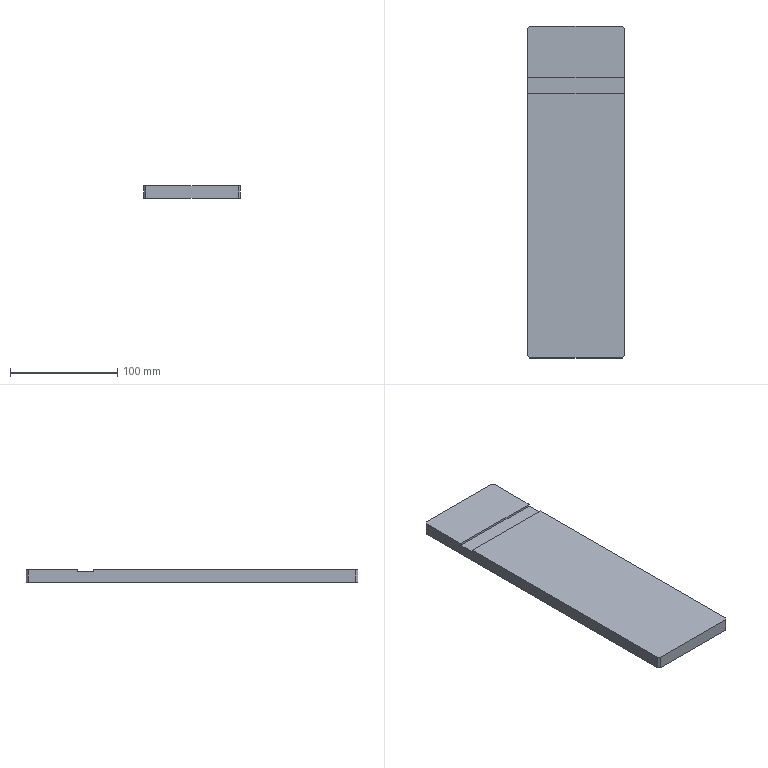Part | STEP file | 001-005-Shaft threading fixture vertical plate | 1 solid | 14 faces | box 90 x 310 x 12 mm | volume 332004 mm3 | plane 14
STEP:
#1=CARTESIAN_POINT('',(0.,0.,0.));
#2=DIRECTION('',(0.,0.,1.));
#3=DIRECTION('',(1.,0.,0.));
#4=AXIS2_PLACEMENT_3D('',#1,#2,#3);
#5=CARTESIAN_POINT('',(-45.,153.,12.));
#6=VERTEX_POINT('',#5);
#7=CARTESIAN_POINT('',(-45.,107.,12.));
#8=VERTEX_POINT('',#7);
#9=CARTESIAN_POINT('',(-45.,-155.,12.));
#10=DIRECTION('',(0.,-1.,0.));
#11=VECTOR('',#10,1.);
#12=LINE('',#9,#11);
#13=CARTESIAN_POINT('',(0.,0.,12.));
#14=DIRECTION('',(0.,0.,-1.));
#15=DIRECTION('',(-1.,0.,0.));
#16=AXIS2_PLACEMENT_3D('',#13,#14,#15);
#17=PLANE('',#16);
#18=CARTESIAN_POINT('',(45.,-155.));
#19=DIRECTION('',(0.,-1.));
#20=VECTOR('',#19,1.);
#21=LINE('',#18,#20);
#22=(GEOMETRIC_REPRESENTATION_CONTEXT(2)PARAMETRIC_REPRESENTATION_CONTEXT()REPRESENTATION_CONTEXT('',''));
#23=DEFINITIONAL_REPRESENTATION('',(#21),#22);
#24=PCURVE('',#17,#23);
#25=CARTESIAN_POINT('',(-45.,-155.,12.));
#26=DIRECTION('',(1.,0.,0.));
#27=DIRECTION('',(0.,1.,0.));
#28=AXIS2_PLACEMENT_3D('',#25,#26,#27);
#29=PLANE('',#28);
#30=CARTESIAN_POINT('',(0.,0.));
#31=DIRECTION('',(-1.,0.));
#32=VECTOR('',#31,1.);
#33=LINE('',#30,#32);
#34=(GEOMETRIC_REPRESENTATION_CONTEXT(2)PARAMETRIC_REPRESENTATION_CONTEXT()REPRESENTATION_CONTEXT('',''));
#35=DEFINITIONAL_REPRESENTATION('',(#33),#34);
#36=PCURVE('',#29,#35);
#37=SURFACE_CURVE('',#12,(#24,#36),.PCURVE_S1.);
#38=EDGE_CURVE('',#6,#8,#37,.T.);
#39=ORIENTED_EDGE('',*,*,#38,.T.);
#40=CARTESIAN_POINT('',(45.,107.,12.));
#41=VERTEX_POINT('',#40);
#42=CARTESIAN_POINT('',(-45.,107.,12.));
#43=DIRECTION('',(1.,0.,0.));
#44=VECTOR('',#43,1.);
#45=LINE('',#42,#44);
#46=CARTESIAN_POINT('',(45.,107.));
#47=DIRECTION('',(-1.,0.));
#48=VECTOR('',#47,1.);
#49=LINE('',#46,#48);
#50=(GEOMETRIC_REPRESENTATION_CONTEXT(2)PARAMETRIC_REPRESENTATION_CONTEXT()REPRESENTATION_CONTEXT('',''));
#51=DEFINITIONAL_REPRESENTATION('',(#49),#50);
#52=PCURVE('',#17,#51);
#53=CARTESIAN_POINT('',(-45.,107.,12.));
#54=DIRECTION('',(0.,1.,0.));
#55=DIRECTION('',(0.,0.,1.));
#56=AXIS2_PLACEMENT_3D('',#53,#54,#55);
#57=PLANE('',#56);
#58=CARTESIAN_POINT('',(0.,0.));
#59=DIRECTION('',(0.,1.));
#60=VECTOR('',#59,1.);
#61=LINE('',#58,#60);
#62=(GEOMETRIC_REPRESENTATION_CONTEXT(2)PARAMETRIC_REPRESENTATION_CONTEXT()REPRESENTATION_CONTEXT('',''));
#63=DEFINITIONAL_REPRESENTATION('',(#61),#62);
#64=PCURVE('',#57,#63);
#65=SURFACE_CURVE('',#45,(#52,#64),.PCURVE_S1.);
#66=EDGE_CURVE('',#8,#41,#65,.T.);
#67=ORIENTED_EDGE('',*,*,#66,.T.);
#68=CARTESIAN_POINT('',(45.,153.,12.));
#69=VERTEX_POINT('',#68);
#70=CARTESIAN_POINT('',(45.,-155.,12.));
#71=DIRECTION('',(0.,1.,0.));
#72=VECTOR('',#71,1.);
#73=LINE('',#70,#72);
#74=CARTESIAN_POINT('',(-45.,-155.));
#75=DIRECTION('',(0.,1.));
#76=VECTOR('',#75,1.);
#77=LINE('',#74,#76);
#78=(GEOMETRIC_REPRESENTATION_CONTEXT(2)PARAMETRIC_REPRESENTATION_CONTEXT()REPRESENTATION_CONTEXT('',''));
#79=DEFINITIONAL_REPRESENTATION('',(#77),#78);
#80=PCURVE('',#17,#79);
#81=CARTESIAN_POINT('',(45.,-155.,12.));
#82=DIRECTION('',(-1.,0.,0.));
#83=DIRECTION('',(0.,-1.,0.));
#84=AXIS2_PLACEMENT_3D('',#81,#82,#83);
#85=PLANE('',#84);
#86=CARTESIAN_POINT('',(0.,0.));
#87=DIRECTION('',(-1.,0.));
#88=VECTOR('',#87,1.);
#89=LINE('',#86,#88);
#90=(GEOMETRIC_REPRESENTATION_CONTEXT(2)PARAMETRIC_REPRESENTATION_CONTEXT()REPRESENTATION_CONTEXT('',''));
#91=DEFINITIONAL_REPRESENTATION('',(#89),#90);
#92=PCURVE('',#85,#91);
#93=SURFACE_CURVE('',#73,(#80,#92),.PCURVE_S1.);
#94=EDGE_CURVE('',#41,#69,#93,.T.);
#95=ORIENTED_EDGE('',*,*,#94,.T.);
#96=CARTESIAN_POINT('',(43.,155.,12.));
#97=VERTEX_POINT('',#96);
#98=CARTESIAN_POINT('',(43.,155.,12.));
#99=DIRECTION('',(-0.7071,0.7071,0.));
#100=VECTOR('',#99,1.);
#101=LINE('',#98,#100);
#102=CARTESIAN_POINT('',(-43.,155.));
#103=DIRECTION('',(0.7071,0.7071));
#104=VECTOR('',#103,1.);
#105=LINE('',#102,#104);
#106=(GEOMETRIC_REPRESENTATION_CONTEXT(2)PARAMETRIC_REPRESENTATION_CONTEXT()REPRESENTATION_CONTEXT('',''));
#107=DEFINITIONAL_REPRESENTATION('',(#105),#106);
#108=PCURVE('',#17,#107);
#109=CARTESIAN_POINT('',(43.,155.,12.));
#110=DIRECTION('',(-0.7071,-0.7071,0.));
#111=DIRECTION('',(0.,0.,-1.));
#112=AXIS2_PLACEMENT_3D('',#109,#110,#111);
#113=PLANE('',#112);
#114=CARTESIAN_POINT('',(0.,0.));
#115=DIRECTION('',(0.,-1.));
#116=VECTOR('',#115,1.);
#117=LINE('',#114,#116);
#118=(GEOMETRIC_REPRESENTATION_CONTEXT(2)PARAMETRIC_REPRESENTATION_CONTEXT()REPRESENTATION_CONTEXT('',''));
#119=DEFINITIONAL_REPRESENTATION('',(#117),#118);
#120=PCURVE('',#113,#119);
#121=SURFACE_CURVE('',#101,(#108,#120),.PCURVE_S1.);
#122=EDGE_CURVE('',#69,#97,#121,.T.);
#123=ORIENTED_EDGE('',*,*,#122,.T.);
#124=CARTESIAN_POINT('',(-43.,155.,12.));
#125=VERTEX_POINT('',#124);
#126=CARTESIAN_POINT('',(-45.,155.,12.));
#127=DIRECTION('',(-1.,0.,0.));
#128=VECTOR('',#127,1.);
#129=LINE('',#126,#128);
#130=CARTESIAN_POINT('',(45.,155.));
#131=DIRECTION('',(1.,0.));
#132=VECTOR('',#131,1.);
#133=LINE('',#130,#132);
#134=(GEOMETRIC_REPRESENTATION_CONTEXT(2)PARAMETRIC_REPRESENTATION_CONTEXT()REPRESENTATION_CONTEXT('',''));
#135=DEFINITIONAL_REPRESENTATION('',(#133),#134);
#136=PCURVE('',#17,#135);
#137=CARTESIAN_POINT('',(-45.,155.,12.));
#138=DIRECTION('',(0.,-1.,0.));
#139=DIRECTION('',(0.,0.,-1.));
#140=AXIS2_PLACEMENT_3D('',#137,#138,#139);
#141=PLANE('',#140);
#142=CARTESIAN_POINT('',(0.,0.));
#143=DIRECTION('',(0.,-1.));
#144=VECTOR('',#143,1.);
#145=LINE('',#142,#144);
#146=(GEOMETRIC_REPRESENTATION_CONTEXT(2)PARAMETRIC_REPRESENTATION_CONTEXT()REPRESENTATION_CONTEXT('',''));
#147=DEFINITIONAL_REPRESENTATION('',(#145),#146);
#148=PCURVE('',#141,#147);
#149=SURFACE_CURVE('',#129,(#136,#148),.PCURVE_S1.);
#150=EDGE_CURVE('',#97,#125,#149,.T.);
#151=ORIENTED_EDGE('',*,*,#150,.T.);
#152=CARTESIAN_POINT('',(-45.,153.,12.));
#153=DIRECTION('',(-0.7071,-0.7071,0.));
#154=VECTOR('',#153,1.);
#155=LINE('',#152,#154);
#156=CARTESIAN_POINT('',(45.,153.));
#157=DIRECTION('',(0.7071,-0.7071));
#158=VECTOR('',#157,1.);
#159=LINE('',#156,#158);
#160=(GEOMETRIC_REPRESENTATION_CONTEXT(2)PARAMETRIC_REPRESENTATION_CONTEXT()REPRESENTATION_CONTEXT('',''));
#161=DEFINITIONAL_REPRESENTATION('',(#159),#160);
#162=PCURVE('',#17,#161);
#163=CARTESIAN_POINT('',(-45.,153.,12.));
#164=DIRECTION('',(0.7071,-0.7071,0.));
#165=DIRECTION('',(0.,0.,-1.));
#166=AXIS2_PLACEMENT_3D('',#163,#164,#165);
#167=PLANE('',#166);
#168=CARTESIAN_POINT('',(0.,0.));
#169=DIRECTION('',(0.,-1.));
#170=VECTOR('',#169,1.);
#171=LINE('',#168,#170);
#172=(GEOMETRIC_REPRESENTATION_CONTEXT(2)PARAMETRIC_REPRESENTATION_CONTEXT()REPRESENTATION_CONTEXT('',''));
#173=DEFINITIONAL_REPRESENTATION('',(#171),#172);
#174=PCURVE('',#167,#173);
#175=SURFACE_CURVE('',#155,(#162,#174),.PCURVE_S1.);
#176=EDGE_CURVE('',#125,#6,#175,.T.);
#177=ORIENTED_EDGE('',*,*,#176,.T.);
#178=EDGE_LOOP('',(#39,#67,#95,#123,#151,#177));
#179=FACE_BOUND('',#178,.T.);
#180=ADVANCED_FACE('',(#179),#17,.F.);
#181=ORIENTED_EDGE('',*,*,#94,.F.);
#182=CARTESIAN_POINT('',(45.,107.,10.));
#183=VERTEX_POINT('',#182);
#184=CARTESIAN_POINT('',(45.,107.,12.));
#185=DIRECTION('',(0.,0.,1.));
#186=VECTOR('',#185,1.);
#187=LINE('',#184,#186);
#188=CARTESIAN_POINT('',(-262.,0.));
#189=DIRECTION('',(0.,1.));
#190=VECTOR('',#189,1.);
#191=LINE('',#188,#190);
#192=(GEOMETRIC_REPRESENTATION_CONTEXT(2)PARAMETRIC_REPRESENTATION_CONTEXT()REPRESENTATION_CONTEXT('',''));
#193=DEFINITIONAL_REPRESENTATION('',(#191),#192);
#194=PCURVE('',#85,#193);
#195=CARTESIAN_POINT('',(0.,90.));
#196=DIRECTION('',(1.,0.));
#197=VECTOR('',#196,1.);
#198=LINE('',#195,#197);
#199=(GEOMETRIC_REPRESENTATION_CONTEXT(2)PARAMETRIC_REPRESENTATION_CONTEXT()REPRESENTATION_CONTEXT('',''));
#200=DEFINITIONAL_REPRESENTATION('',(#198),#199);
#201=PCURVE('',#57,#200);
#202=SURFACE_CURVE('',#187,(#194,#201),.PCURVE_S1.);
#203=EDGE_CURVE('',#183,#41,#202,.T.);
#204=ORIENTED_EDGE('',*,*,#203,.F.);
#205=CARTESIAN_POINT('',(45.,92.,10.));
#206=VERTEX_POINT('',#205);
#207=CARTESIAN_POINT('',(45.,107.,10.));
#208=DIRECTION('',(0.,1.,0.));
#209=VECTOR('',#208,1.);
#210=LINE('',#207,#209);
#211=CARTESIAN_POINT('',(-262.,-2.));
#212=DIRECTION('',(-1.,0.));
#213=VECTOR('',#212,1.);
#214=LINE('',#211,#213);
#215=(GEOMETRIC_REPRESENTATION_CONTEXT(2)PARAMETRIC_REPRESENTATION_CONTEXT()REPRESENTATION_CONTEXT('',''));
#216=DEFINITIONAL_REPRESENTATION('',(#214),#215);
#217=PCURVE('',#85,#216);
#218=CARTESIAN_POINT('',(-45.,107.,10.));
#219=DIRECTION('',(0.,0.,-1.));
#220=DIRECTION('',(0.,1.,0.));
#221=AXIS2_PLACEMENT_3D('',#218,#219,#220);
#222=PLANE('',#221);
#223=CARTESIAN_POINT('',(0.,90.));
#224=DIRECTION('',(1.,0.));
#225=VECTOR('',#224,1.);
#226=LINE('',#223,#225);
#227=(GEOMETRIC_REPRESENTATION_CONTEXT(2)PARAMETRIC_REPRESENTATION_CONTEXT()REPRESENTATION_CONTEXT('',''));
#228=DEFINITIONAL_REPRESENTATION('',(#226),#227);
#229=PCURVE('',#222,#228);
#230=SURFACE_CURVE('',#210,(#217,#229),.PCURVE_S1.);
#231=EDGE_CURVE('',#206,#183,#230,.T.);
#232=ORIENTED_EDGE('',*,*,#231,.F.);
#233=CARTESIAN_POINT('',(45.,92.,12.));
#234=VERTEX_POINT('',#233);
#235=CARTESIAN_POINT('',(45.,92.,12.));
#236=DIRECTION('',(0.,0.,-1.));
#237=VECTOR('',#236,1.);
#238=LINE('',#235,#237);
#239=CARTESIAN_POINT('',(-247.,0.));
#240=DIRECTION('',(0.,-1.));
#241=VECTOR('',#240,1.);
#242=LINE('',#239,#241);
#243=(GEOMETRIC_REPRESENTATION_CONTEXT(2)PARAMETRIC_REPRESENTATION_CONTEXT()REPRESENTATION_CONTEXT('',''));
#244=DEFINITIONAL_REPRESENTATION('',(#242),#243);
#245=PCURVE('',#85,#244);
#246=CARTESIAN_POINT('',(-45.,92.,12.));
#247=DIRECTION('',(0.,-1.,0.));
#248=DIRECTION('',(1.,0.,0.));
#249=AXIS2_PLACEMENT_3D('',#246,#247,#248);
#250=PLANE('',#249);
#251=CARTESIAN_POINT('',(90.,0.));
#252=DIRECTION('',(0.,-1.));
#253=VECTOR('',#252,1.);
#254=LINE('',#251,#253);
#255=(GEOMETRIC_REPRESENTATION_CONTEXT(2)PARAMETRIC_REPRESENTATION_CONTEXT()REPRESENTATION_CONTEXT('',''));
#256=DEFINITIONAL_REPRESENTATION('',(#254),#255);
#257=PCURVE('',#250,#256);
#258=SURFACE_CURVE('',#238,(#245,#257),.PCURVE_S1.);
#259=EDGE_CURVE('',#234,#206,#258,.T.);
#260=ORIENTED_EDGE('',*,*,#259,.F.);
#261=CARTESIAN_POINT('',(45.,-153.,12.));
#262=VERTEX_POINT('',#261);
#263=CARTESIAN_POINT('',(45.,-155.,12.));
#264=DIRECTION('',(0.,1.,0.));
#265=VECTOR('',#264,1.);
#266=LINE('',#263,#265);
#267=CARTESIAN_POINT('',(0.,0.));
#268=DIRECTION('',(-1.,0.));
#269=VECTOR('',#268,1.);
#270=LINE('',#267,#269);
#271=(GEOMETRIC_REPRESENTATION_CONTEXT(2)PARAMETRIC_REPRESENTATION_CONTEXT()REPRESENTATION_CONTEXT('',''));
#272=DEFINITIONAL_REPRESENTATION('',(#270),#271);
#273=PCURVE('',#85,#272);
#274=CARTESIAN_POINT('',(0.,0.,12.));
#275=DIRECTION('',(0.,0.,-1.));
#276=DIRECTION('',(-1.,0.,0.));
#277=AXIS2_PLACEMENT_3D('',#274,#275,#276);
#278=PLANE('',#277);
#279=CARTESIAN_POINT('',(-45.,-155.));
#280=DIRECTION('',(0.,1.));
#281=VECTOR('',#280,1.);
#282=LINE('',#279,#281);
#283=(GEOMETRIC_REPRESENTATION_CONTEXT(2)PARAMETRIC_REPRESENTATION_CONTEXT()REPRESENTATION_CONTEXT('',''));
#284=DEFINITIONAL_REPRESENTATION('',(#282),#283);
#285=PCURVE('',#278,#284);
#286=SURFACE_CURVE('',#266,(#273,#285),.PCURVE_S1.);
#287=EDGE_CURVE('',#262,#234,#286,.T.);
#288=ORIENTED_EDGE('',*,*,#287,.F.);
#289=CARTESIAN_POINT('',(45.,-153.,0.));
#290=VERTEX_POINT('',#289);
#291=CARTESIAN_POINT('',(45.,-153.,12.));
#292=DIRECTION('',(0.,0.,-1.));
#293=VECTOR('',#292,1.);
#294=LINE('',#291,#293);
#295=CARTESIAN_POINT('',(-2.,0.));
#296=DIRECTION('',(0.,-1.));
#297=VECTOR('',#296,1.);
#298=LINE('',#295,#297);
#299=(GEOMETRIC_REPRESENTATION_CONTEXT(2)PARAMETRIC_REPRESENTATION_CONTEXT()REPRESENTATION_CONTEXT('',''));
#300=DEFINITIONAL_REPRESENTATION('',(#298),#299);
#301=PCURVE('',#85,#300);
#302=CARTESIAN_POINT('',(45.,-153.,12.));
#303=DIRECTION('',(-0.7071,0.7071,0.));
#304=DIRECTION('',(0.,0.,-1.));
#305=AXIS2_PLACEMENT_3D('',#302,#303,#304);
#306=PLANE('',#305);
#307=CARTESIAN_POINT('',(0.,0.));
#308=DIRECTION('',(1.,0.));
#309=VECTOR('',#308,1.);
#310=LINE('',#307,#309);
#311=(GEOMETRIC_REPRESENTATION_CONTEXT(2)PARAMETRIC_REPRESENTATION_CONTEXT()REPRESENTATION_CONTEXT('',''));
#312=DEFINITIONAL_REPRESENTATION('',(#310),#311);
#313=PCURVE('',#306,#312);
#314=SURFACE_CURVE('',#294,(#301,#313),.PCURVE_S1.);
#315=EDGE_CURVE('',#262,#290,#314,.T.);
#316=ORIENTED_EDGE('',*,*,#315,.T.);
#317=CARTESIAN_POINT('',(45.,153.,0.));
#318=VERTEX_POINT('',#317);
#319=CARTESIAN_POINT('',(45.,-155.,0.));
#320=DIRECTION('',(0.,1.,0.));
#321=VECTOR('',#320,1.);
#322=LINE('',#319,#321);
#323=CARTESIAN_POINT('',(0.,-12.));
#324=DIRECTION('',(-1.,0.));
#325=VECTOR('',#324,1.);
#326=LINE('',#323,#325);
#327=(GEOMETRIC_REPRESENTATION_CONTEXT(2)PARAMETRIC_REPRESENTATION_CONTEXT()REPRESENTATION_CONTEXT('',''));
#328=DEFINITIONAL_REPRESENTATION('',(#326),#327);
#329=PCURVE('',#85,#328);
#330=CARTESIAN_POINT('',(0.,0.,0.));
#331=DIRECTION('',(0.,0.,-1.));
#332=DIRECTION('',(-1.,0.,0.));
#333=AXIS2_PLACEMENT_3D('',#330,#331,#332);
#334=PLANE('',#333);
#335=CARTESIAN_POINT('',(-45.,-155.));
#336=DIRECTION('',(0.,1.));
#337=VECTOR('',#336,1.);
#338=LINE('',#335,#337);
#339=(GEOMETRIC_REPRESENTATION_CONTEXT(2)PARAMETRIC_REPRESENTATION_CONTEXT()REPRESENTATION_CONTEXT('',''));
#340=DEFINITIONAL_REPRESENTATION('',(#338),#339);
#341=PCURVE('',#334,#340);
#342=SURFACE_CURVE('',#322,(#329,#341),.PCURVE_S1.);
#343=EDGE_CURVE('',#290,#318,#342,.T.);
#344=ORIENTED_EDGE('',*,*,#343,.T.);
#345=CARTESIAN_POINT('',(45.,153.,12.));
#346=DIRECTION('',(0.,0.,1.));
#347=VECTOR('',#346,1.);
#348=LINE('',#345,#347);
#349=CARTESIAN_POINT('',(-308.,0.));
#350=DIRECTION('',(0.,1.));
#351=VECTOR('',#350,1.);
#352=LINE('',#349,#351);
#353=(GEOMETRIC_REPRESENTATION_CONTEXT(2)PARAMETRIC_REPRESENTATION_CONTEXT()REPRESENTATION_CONTEXT('',''));
#354=DEFINITIONAL_REPRESENTATION('',(#352),#353);
#355=PCURVE('',#85,#354);
#356=CARTESIAN_POINT('',(0.,2.828));
#357=DIRECTION('',(-1.,0.));
#358=VECTOR('',#357,1.);
#359=LINE('',#356,#358);
#360=(GEOMETRIC_REPRESENTATION_CONTEXT(2)PARAMETRIC_REPRESENTATION_CONTEXT()REPRESENTATION_CONTEXT('',''));
#361=DEFINITIONAL_REPRESENTATION('',(#359),#360);
#362=PCURVE('',#113,#361);
#363=SURFACE_CURVE('',#348,(#355,#362),.PCURVE_S1.);
#364=EDGE_CURVE('',#318,#69,#363,.T.);
#365=ORIENTED_EDGE('',*,*,#364,.T.);
#366=EDGE_LOOP('',(#181,#204,#232,#260,#288,#316,#344,#365));
#367=FACE_BOUND('',#366,.T.);
#368=ADVANCED_FACE('',(#367),#85,.F.);
#369=CARTESIAN_POINT('',(43.,155.,0.));
#370=VERTEX_POINT('',#369);
#371=CARTESIAN_POINT('',(-43.,155.,0.));
#372=VERTEX_POINT('',#371);
#373=CARTESIAN_POINT('',(-45.,155.,0.));
#374=DIRECTION('',(-1.,0.,0.));
#375=VECTOR('',#374,1.);
#376=LINE('',#373,#375);
#377=CARTESIAN_POINT('',(12.,0.));
#378=DIRECTION('',(0.,-1.));
#379=VECTOR('',#378,1.);
#380=LINE('',#377,#379);
#381=(GEOMETRIC_REPRESENTATION_CONTEXT(2)PARAMETRIC_REPRESENTATION_CONTEXT()REPRESENTATION_CONTEXT('',''));
#382=DEFINITIONAL_REPRESENTATION('',(#380),#381);
#383=PCURVE('',#141,#382);
#384=CARTESIAN_POINT('',(45.,155.));
#385=DIRECTION('',(1.,0.));
#386=VECTOR('',#385,1.);
#387=LINE('',#384,#386);
#388=(GEOMETRIC_REPRESENTATION_CONTEXT(2)PARAMETRIC_REPRESENTATION_CONTEXT()REPRESENTATION_CONTEXT('',''));
#389=DEFINITIONAL_REPRESENTATION('',(#387),#388);
#390=PCURVE('',#334,#389);
#391=SURFACE_CURVE('',#376,(#383,#390),.PCURVE_S1.);
#392=EDGE_CURVE('',#370,#372,#391,.T.);
#393=ORIENTED_EDGE('',*,*,#392,.T.);
#394=CARTESIAN_POINT('',(-43.,155.,12.));
#395=DIRECTION('',(0.,0.,1.));
#396=VECTOR('',#395,1.);
#397=LINE('',#394,#396);
#398=CARTESIAN_POINT('',(0.,2.));
#399=DIRECTION('',(-1.,0.));
#400=VECTOR('',#399,1.);
#401=LINE('',#398,#400);
#402=(GEOMETRIC_REPRESENTATION_CONTEXT(2)PARAMETRIC_REPRESENTATION_CONTEXT()REPRESENTATION_CONTEXT('',''));
#403=DEFINITIONAL_REPRESENTATION('',(#401),#402);
#404=PCURVE('',#141,#403);
#405=CARTESIAN_POINT('',(0.,2.828));
#406=DIRECTION('',(-1.,0.));
#407=VECTOR('',#406,1.);
#408=LINE('',#405,#407);
#409=(GEOMETRIC_REPRESENTATION_CONTEXT(2)PARAMETRIC_REPRESENTATION_CONTEXT()REPRESENTATION_CONTEXT('',''));
#410=DEFINITIONAL_REPRESENTATION('',(#408),#409);
#411=PCURVE('',#167,#410);
#412=SURFACE_CURVE('',#397,(#404,#411),.PCURVE_S1.);
#413=EDGE_CURVE('',#372,#125,#412,.T.);
#414=ORIENTED_EDGE('',*,*,#413,.T.);
#415=ORIENTED_EDGE('',*,*,#150,.F.);
#416=CARTESIAN_POINT('',(43.,155.,12.));
#417=DIRECTION('',(0.,0.,-1.));
#418=VECTOR('',#417,1.);
#419=LINE('',#416,#418);
#420=CARTESIAN_POINT('',(0.,88.));
#421=DIRECTION('',(1.,0.));
#422=VECTOR('',#421,1.);
#423=LINE('',#420,#422);
#424=(GEOMETRIC_REPRESENTATION_CONTEXT(2)PARAMETRIC_REPRESENTATION_CONTEXT()REPRESENTATION_CONTEXT('',''));
#425=DEFINITIONAL_REPRESENTATION('',(#423),#424);
#426=PCURVE('',#141,#425);
#427=CARTESIAN_POINT('',(0.,0.));
#428=DIRECTION('',(1.,0.));
#429=VECTOR('',#428,1.);
#430=LINE('',#427,#429);
#431=(GEOMETRIC_REPRESENTATION_CONTEXT(2)PARAMETRIC_REPRESENTATION_CONTEXT()REPRESENTATION_CONTEXT('',''));
#432=DEFINITIONAL_REPRESENTATION('',(#430),#431);
#433=PCURVE('',#113,#432);
#434=SURFACE_CURVE('',#419,(#426,#433),.PCURVE_S1.);
#435=EDGE_CURVE('',#97,#370,#434,.T.);
#436=ORIENTED_EDGE('',*,*,#435,.T.);
#437=EDGE_LOOP('',(#393,#414,#415,#436));
#438=FACE_BOUND('',#437,.T.);
#439=ADVANCED_FACE('',(#438),#141,.F.);
#440=CARTESIAN_POINT('',(-45.,92.,10.));
#441=VERTEX_POINT('',#440);
#442=CARTESIAN_POINT('',(-45.,107.,10.));
#443=VERTEX_POINT('',#442);
#444=CARTESIAN_POINT('',(-45.,107.,10.));
#445=DIRECTION('',(0.,1.,0.));
#446=VECTOR('',#445,1.);
#447=LINE('',#444,#446);
#448=CARTESIAN_POINT('',(262.,-2.));
#449=DIRECTION('',(1.,0.));
#450=VECTOR('',#449,1.);
#451=LINE('',#448,#450);
#452=(GEOMETRIC_REPRESENTATION_CONTEXT(2)PARAMETRIC_REPRESENTATION_CONTEXT()REPRESENTATION_CONTEXT('',''));
#453=DEFINITIONAL_REPRESENTATION('',(#451),#452);
#454=PCURVE('',#29,#453);
#455=CARTESIAN_POINT('',(0.,0.));
#456=DIRECTION('',(1.,0.));
#457=VECTOR('',#456,1.);
#458=LINE('',#455,#457);
#459=(GEOMETRIC_REPRESENTATION_CONTEXT(2)PARAMETRIC_REPRESENTATION_CONTEXT()REPRESENTATION_CONTEXT('',''));
#460=DEFINITIONAL_REPRESENTATION('',(#458),#459);
#461=PCURVE('',#222,#460);
#462=SURFACE_CURVE('',#447,(#454,#461),.PCURVE_S1.);
#463=EDGE_CURVE('',#441,#443,#462,.T.);
#464=ORIENTED_EDGE('',*,*,#463,.T.);
#465=CARTESIAN_POINT('',(-45.,107.,12.));
#466=DIRECTION('',(0.,0.,1.));
#467=VECTOR('',#466,1.);
#468=LINE('',#465,#467);
#469=CARTESIAN_POINT('',(262.,0.));
#470=DIRECTION('',(0.,1.));
#471=VECTOR('',#470,1.);
#472=LINE('',#469,#471);
#473=(GEOMETRIC_REPRESENTATION_CONTEXT(2)PARAMETRIC_REPRESENTATION_CONTEXT()REPRESENTATION_CONTEXT('',''));
#474=DEFINITIONAL_REPRESENTATION('',(#472),#473);
#475=PCURVE('',#29,#474);
#476=CARTESIAN_POINT('',(0.,0.));
#477=DIRECTION('',(1.,0.));
#478=VECTOR('',#477,1.);
#479=LINE('',#476,#478);
#480=(GEOMETRIC_REPRESENTATION_CONTEXT(2)PARAMETRIC_REPRESENTATION_CONTEXT()REPRESENTATION_CONTEXT('',''));
#481=DEFINITIONAL_REPRESENTATION('',(#479),#480);
#482=PCURVE('',#57,#481);
#483=SURFACE_CURVE('',#468,(#475,#482),.PCURVE_S1.);
#484=EDGE_CURVE('',#443,#8,#483,.T.);
#485=ORIENTED_EDGE('',*,*,#484,.T.);
#486=ORIENTED_EDGE('',*,*,#38,.F.);
#487=CARTESIAN_POINT('',(-45.,153.,0.));
#488=VERTEX_POINT('',#487);
#489=CARTESIAN_POINT('',(-45.,153.,12.));
#490=DIRECTION('',(0.,0.,-1.));
#491=VECTOR('',#490,1.);
#492=LINE('',#489,#491);
#493=CARTESIAN_POINT('',(308.,0.));
#494=DIRECTION('',(0.,-1.));
#495=VECTOR('',#494,1.);
#496=LINE('',#493,#495);
#497=(GEOMETRIC_REPRESENTATION_CONTEXT(2)PARAMETRIC_REPRESENTATION_CONTEXT()REPRESENTATION_CONTEXT('',''));
#498=DEFINITIONAL_REPRESENTATION('',(#496),#497);
#499=PCURVE('',#29,#498);
#500=CARTESIAN_POINT('',(0.,0.));
#501=DIRECTION('',(1.,0.));
#502=VECTOR('',#501,1.);
#503=LINE('',#500,#502);
#504=(GEOMETRIC_REPRESENTATION_CONTEXT(2)PARAMETRIC_REPRESENTATION_CONTEXT()REPRESENTATION_CONTEXT('',''));
#505=DEFINITIONAL_REPRESENTATION('',(#503),#504);
#506=PCURVE('',#167,#505);
#507=SURFACE_CURVE('',#492,(#499,#506),.PCURVE_S1.);
#508=EDGE_CURVE('',#6,#488,#507,.T.);
#509=ORIENTED_EDGE('',*,*,#508,.T.);
#510=CARTESIAN_POINT('',(-45.,-153.,0.));
#511=VERTEX_POINT('',#510);
#512=CARTESIAN_POINT('',(-45.,-155.,0.));
#513=DIRECTION('',(0.,-1.,0.));
#514=VECTOR('',#513,1.);
#515=LINE('',#512,#514);
#516=CARTESIAN_POINT('',(0.,-12.));
#517=DIRECTION('',(-1.,0.));
#518=VECTOR('',#517,1.);
#519=LINE('',#516,#518);
#520=(GEOMETRIC_REPRESENTATION_CONTEXT(2)PARAMETRIC_REPRESENTATION_CONTEXT()REPRESENTATION_CONTEXT('',''));
#521=DEFINITIONAL_REPRESENTATION('',(#519),#520);
#522=PCURVE('',#29,#521);
#523=CARTESIAN_POINT('',(45.,-155.));
#524=DIRECTION('',(0.,-1.));
#525=VECTOR('',#524,1.);
#526=LINE('',#523,#525);
#527=(GEOMETRIC_REPRESENTATION_CONTEXT(2)PARAMETRIC_REPRESENTATION_CONTEXT()REPRESENTATION_CONTEXT('',''));
#528=DEFINITIONAL_REPRESENTATION('',(#526),#527);
#529=PCURVE('',#334,#528);
#530=SURFACE_CURVE('',#515,(#522,#529),.PCURVE_S1.);
#531=EDGE_CURVE('',#488,#511,#530,.T.);
#532=ORIENTED_EDGE('',*,*,#531,.T.);
#533=CARTESIAN_POINT('',(-45.,-153.,12.));
#534=VERTEX_POINT('',#533);
#535=CARTESIAN_POINT('',(-45.,-153.,12.));
#536=DIRECTION('',(0.,0.,1.));
#537=VECTOR('',#536,1.);
#538=LINE('',#535,#537);
#539=CARTESIAN_POINT('',(2.,0.));
#540=DIRECTION('',(0.,1.));
#541=VECTOR('',#540,1.);
#542=LINE('',#539,#541);
#543=(GEOMETRIC_REPRESENTATION_CONTEXT(2)PARAMETRIC_REPRESENTATION_CONTEXT()REPRESENTATION_CONTEXT('',''));
#544=DEFINITIONAL_REPRESENTATION('',(#542),#543);
#545=PCURVE('',#29,#544);
#546=CARTESIAN_POINT('',(-43.,-155.,12.));
#547=DIRECTION('',(0.7071,0.7071,0.));
#548=DIRECTION('',(0.,0.,-1.));
#549=AXIS2_PLACEMENT_3D('',#546,#547,#548);
#550=PLANE('',#549);
#551=CARTESIAN_POINT('',(0.,2.828));
#552=DIRECTION('',(-1.,0.));
#553=VECTOR('',#552,1.);
#554=LINE('',#551,#553);
#555=(GEOMETRIC_REPRESENTATION_CONTEXT(2)PARAMETRIC_REPRESENTATION_CONTEXT()REPRESENTATION_CONTEXT('',''));
#556=DEFINITIONAL_REPRESENTATION('',(#554),#555);
#557=PCURVE('',#550,#556);
#558=SURFACE_CURVE('',#538,(#545,#557),.PCURVE_S1.);
#559=EDGE_CURVE('',#511,#534,#558,.T.);
#560=ORIENTED_EDGE('',*,*,#559,.T.);
#561=CARTESIAN_POINT('',(-45.,92.,12.));
#562=VERTEX_POINT('',#561);
#563=CARTESIAN_POINT('',(-45.,-155.,12.));
#564=DIRECTION('',(0.,-1.,0.));
#565=VECTOR('',#564,1.);
#566=LINE('',#563,#565);
#567=CARTESIAN_POINT('',(0.,0.));
#568=DIRECTION('',(-1.,0.));
#569=VECTOR('',#568,1.);
#570=LINE('',#567,#569);
#571=(GEOMETRIC_REPRESENTATION_CONTEXT(2)PARAMETRIC_REPRESENTATION_CONTEXT()REPRESENTATION_CONTEXT('',''));
#572=DEFINITIONAL_REPRESENTATION('',(#570),#571);
#573=PCURVE('',#29,#572);
#574=CARTESIAN_POINT('',(45.,-155.));
#575=DIRECTION('',(0.,-1.));
#576=VECTOR('',#575,1.);
#577=LINE('',#574,#576);
#578=(GEOMETRIC_REPRESENTATION_CONTEXT(2)PARAMETRIC_REPRESENTATION_CONTEXT()REPRESENTATION_CONTEXT('',''));
#579=DEFINITIONAL_REPRESENTATION('',(#577),#578);
#580=PCURVE('',#278,#579);
#581=SURFACE_CURVE('',#566,(#573,#580),.PCURVE_S1.);
#582=EDGE_CURVE('',#562,#534,#581,.T.);
#583=ORIENTED_EDGE('',*,*,#582,.F.);
#584=CARTESIAN_POINT('',(-45.,92.,12.));
#585=DIRECTION('',(0.,0.,-1.));
#586=VECTOR('',#585,1.);
#587=LINE('',#584,#586);
#588=CARTESIAN_POINT('',(247.,0.));
#589=DIRECTION('',(0.,-1.));
#590=VECTOR('',#589,1.);
#591=LINE('',#588,#590);
#592=(GEOMETRIC_REPRESENTATION_CONTEXT(2)PARAMETRIC_REPRESENTATION_CONTEXT()REPRESENTATION_CONTEXT('',''));
#593=DEFINITIONAL_REPRESENTATION('',(#591),#592);
#594=PCURVE('',#29,#593);
#595=CARTESIAN_POINT('',(0.,0.));
#596=DIRECTION('',(0.,-1.));
#597=VECTOR('',#596,1.);
#598=LINE('',#595,#597);
#599=(GEOMETRIC_REPRESENTATION_CONTEXT(2)PARAMETRIC_REPRESENTATION_CONTEXT()REPRESENTATION_CONTEXT('',''));
#600=DEFINITIONAL_REPRESENTATION('',(#598),#599);
#601=PCURVE('',#250,#600);
#602=SURFACE_CURVE('',#587,(#594,#601),.PCURVE_S1.);
#603=EDGE_CURVE('',#562,#441,#602,.T.);
#604=ORIENTED_EDGE('',*,*,#603,.T.);
#605=EDGE_LOOP('',(#464,#485,#486,#509,#532,#560,#583,#604));
#606=FACE_BOUND('',#605,.T.);
#607=ADVANCED_FACE('',(#606),#29,.F.);
#608=CARTESIAN_POINT('',(-43.,-155.,0.));
#609=VERTEX_POINT('',#608);
#610=CARTESIAN_POINT('',(43.,-155.,0.));
#611=VERTEX_POINT('',#610);
#612=CARTESIAN_POINT('',(-45.,-155.,0.));
#613=DIRECTION('',(1.,0.,0.));
#614=VECTOR('',#613,1.);
#615=LINE('',#612,#614);
#616=CARTESIAN_POINT('',(-45.,-155.,12.));
#617=DIRECTION('',(0.,1.,0.));
#618=DIRECTION('',(0.,0.,1.));
#619=AXIS2_PLACEMENT_3D('',#616,#617,#618);
#620=PLANE('',#619);
#621=CARTESIAN_POINT('',(-12.,0.));
#622=DIRECTION('',(0.,1.));
#623=VECTOR('',#622,1.);
#624=LINE('',#621,#623);
#625=(GEOMETRIC_REPRESENTATION_CONTEXT(2)PARAMETRIC_REPRESENTATION_CONTEXT()REPRESENTATION_CONTEXT('',''));
#626=DEFINITIONAL_REPRESENTATION('',(#624),#625);
#627=PCURVE('',#620,#626);
#628=CARTESIAN_POINT('',(45.,-155.));
#629=DIRECTION('',(-1.,0.));
#630=VECTOR('',#629,1.);
#631=LINE('',#628,#630);
#632=(GEOMETRIC_REPRESENTATION_CONTEXT(2)PARAMETRIC_REPRESENTATION_CONTEXT()REPRESENTATION_CONTEXT('',''));
#633=DEFINITIONAL_REPRESENTATION('',(#631),#632);
#634=PCURVE('',#334,#633);
#635=SURFACE_CURVE('',#615,(#627,#634),.PCURVE_S1.);
#636=EDGE_CURVE('',#609,#611,#635,.T.);
#637=ORIENTED_EDGE('',*,*,#636,.T.);
#638=CARTESIAN_POINT('',(43.,-155.,12.));
#639=VERTEX_POINT('',#638);
#640=CARTESIAN_POINT('',(43.,-155.,12.));
#641=DIRECTION('',(0.,0.,1.));
#642=VECTOR('',#641,1.);
#643=LINE('',#640,#642);
#644=CARTESIAN_POINT('',(0.,88.));
#645=DIRECTION('',(1.,0.));
#646=VECTOR('',#645,1.);
#647=LINE('',#644,#646);
#648=(GEOMETRIC_REPRESENTATION_CONTEXT(2)PARAMETRIC_REPRESENTATION_CONTEXT()REPRESENTATION_CONTEXT('',''));
#649=DEFINITIONAL_REPRESENTATION('',(#647),#648);
#650=PCURVE('',#620,#649);
#651=CARTESIAN_POINT('',(0.,2.828));
#652=DIRECTION('',(-1.,0.));
#653=VECTOR('',#652,1.);
#654=LINE('',#651,#653);
#655=(GEOMETRIC_REPRESENTATION_CONTEXT(2)PARAMETRIC_REPRESENTATION_CONTEXT()REPRESENTATION_CONTEXT('',''));
#656=DEFINITIONAL_REPRESENTATION('',(#654),#655);
#657=PCURVE('',#306,#656);
#658=SURFACE_CURVE('',#643,(#650,#657),.PCURVE_S1.);
#659=EDGE_CURVE('',#611,#639,#658,.T.);
#660=ORIENTED_EDGE('',*,*,#659,.T.);
#661=CARTESIAN_POINT('',(-43.,-155.,12.));
#662=VERTEX_POINT('',#661);
#663=CARTESIAN_POINT('',(-45.,-155.,12.));
#664=DIRECTION('',(1.,0.,0.));
#665=VECTOR('',#664,1.);
#666=LINE('',#663,#665);
#667=CARTESIAN_POINT('',(0.,0.));
#668=DIRECTION('',(0.,1.));
#669=VECTOR('',#668,1.);
#670=LINE('',#667,#669);
#671=(GEOMETRIC_REPRESENTATION_CONTEXT(2)PARAMETRIC_REPRESENTATION_CONTEXT()REPRESENTATION_CONTEXT('',''));
#672=DEFINITIONAL_REPRESENTATION('',(#670),#671);
#673=PCURVE('',#620,#672);
#674=CARTESIAN_POINT('',(45.,-155.));
#675=DIRECTION('',(-1.,0.));
#676=VECTOR('',#675,1.);
#677=LINE('',#674,#676);
#678=(GEOMETRIC_REPRESENTATION_CONTEXT(2)PARAMETRIC_REPRESENTATION_CONTEXT()REPRESENTATION_CONTEXT('',''));
#679=DEFINITIONAL_REPRESENTATION('',(#677),#678);
#680=PCURVE('',#278,#679);
#681=SURFACE_CURVE('',#666,(#673,#680),.PCURVE_S1.);
#682=EDGE_CURVE('',#662,#639,#681,.T.);
#683=ORIENTED_EDGE('',*,*,#682,.F.);
#684=CARTESIAN_POINT('',(-43.,-155.,12.));
#685=DIRECTION('',(0.,0.,-1.));
#686=VECTOR('',#685,1.);
#687=LINE('',#684,#686);
#688=CARTESIAN_POINT('',(0.,2.));
#689=DIRECTION('',(-1.,0.));
#690=VECTOR('',#689,1.);
#691=LINE('',#688,#690);
#692=(GEOMETRIC_REPRESENTATION_CONTEXT(2)PARAMETRIC_REPRESENTATION_CONTEXT()REPRESENTATION_CONTEXT('',''));
#693=DEFINITIONAL_REPRESENTATION('',(#691),#692);
#694=PCURVE('',#620,#693);
#695=CARTESIAN_POINT('',(0.,0.));
#696=DIRECTION('',(1.,0.));
#697=VECTOR('',#696,1.);
#698=LINE('',#695,#697);
#699=(GEOMETRIC_REPRESENTATION_CONTEXT(2)PARAMETRIC_REPRESENTATION_CONTEXT()REPRESENTATION_CONTEXT('',''));
#700=DEFINITIONAL_REPRESENTATION('',(#698),#699);
#701=PCURVE('',#550,#700);
#702=SURFACE_CURVE('',#687,(#694,#701),.PCURVE_S1.);
#703=EDGE_CURVE('',#662,#609,#702,.T.);
#704=ORIENTED_EDGE('',*,*,#703,.T.);
#705=EDGE_LOOP('',(#637,#660,#683,#704));
#706=FACE_BOUND('',#705,.T.);
#707=ADVANCED_FACE('',(#706),#620,.F.);
#708=ORIENTED_EDGE('',*,*,#287,.T.);
#709=CARTESIAN_POINT('',(-45.,92.,12.));
#710=DIRECTION('',(1.,0.,0.));
#711=VECTOR('',#710,1.);
#712=LINE('',#709,#711);
#713=CARTESIAN_POINT('',(45.,92.));
#714=DIRECTION('',(-1.,0.));
#715=VECTOR('',#714,1.);
#716=LINE('',#713,#715);
#717=(GEOMETRIC_REPRESENTATION_CONTEXT(2)PARAMETRIC_REPRESENTATION_CONTEXT()REPRESENTATION_CONTEXT('',''));
#718=DEFINITIONAL_REPRESENTATION('',(#716),#717);
#719=PCURVE('',#278,#718);
#720=CARTESIAN_POINT('',(0.,0.));
#721=DIRECTION('',(1.,0.));
#722=VECTOR('',#721,1.);
#723=LINE('',#720,#722);
#724=(GEOMETRIC_REPRESENTATION_CONTEXT(2)PARAMETRIC_REPRESENTATION_CONTEXT()REPRESENTATION_CONTEXT('',''));
#725=DEFINITIONAL_REPRESENTATION('',(#723),#724);
#726=PCURVE('',#250,#725);
#727=SURFACE_CURVE('',#712,(#719,#726),.PCURVE_S1.);
#728=EDGE_CURVE('',#562,#234,#727,.T.);
#729=ORIENTED_EDGE('',*,*,#728,.F.);
#730=ORIENTED_EDGE('',*,*,#582,.T.);
#731=CARTESIAN_POINT('',(-43.,-155.,12.));
#732=DIRECTION('',(0.7071,-0.7071,0.));
#733=VECTOR('',#732,1.);
#734=LINE('',#731,#733);
#735=CARTESIAN_POINT('',(43.,-155.));
#736=DIRECTION('',(-0.7071,-0.7071));
#737=VECTOR('',#736,1.);
#738=LINE('',#735,#737);
#739=(GEOMETRIC_REPRESENTATION_CONTEXT(2)PARAMETRIC_REPRESENTATION_CONTEXT()REPRESENTATION_CONTEXT('',''));
#740=DEFINITIONAL_REPRESENTATION('',(#738),#739);
#741=PCURVE('',#278,#740);
#742=CARTESIAN_POINT('',(0.,0.));
#743=DIRECTION('',(0.,-1.));
#744=VECTOR('',#743,1.);
#745=LINE('',#742,#744);
#746=(GEOMETRIC_REPRESENTATION_CONTEXT(2)PARAMETRIC_REPRESENTATION_CONTEXT()REPRESENTATION_CONTEXT('',''));
#747=DEFINITIONAL_REPRESENTATION('',(#745),#746);
#748=PCURVE('',#550,#747);
#749=SURFACE_CURVE('',#734,(#741,#748),.PCURVE_S1.);
#750=EDGE_CURVE('',#534,#662,#749,.T.);
#751=ORIENTED_EDGE('',*,*,#750,.T.);
#752=ORIENTED_EDGE('',*,*,#682,.T.);
#753=CARTESIAN_POINT('',(45.,-153.,12.));
#754=DIRECTION('',(0.7071,0.7071,0.));
#755=VECTOR('',#754,1.);
#756=LINE('',#753,#755);
#757=CARTESIAN_POINT('',(-45.,-153.));
#758=DIRECTION('',(-0.7071,0.7071));
#759=VECTOR('',#758,1.);
#760=LINE('',#757,#759);
#761=(GEOMETRIC_REPRESENTATION_CONTEXT(2)PARAMETRIC_REPRESENTATION_CONTEXT()REPRESENTATION_CONTEXT('',''));
#762=DEFINITIONAL_REPRESENTATION('',(#760),#761);
#763=PCURVE('',#278,#762);
#764=CARTESIAN_POINT('',(0.,0.));
#765=DIRECTION('',(0.,-1.));
#766=VECTOR('',#765,1.);
#767=LINE('',#764,#766);
#768=(GEOMETRIC_REPRESENTATION_CONTEXT(2)PARAMETRIC_REPRESENTATION_CONTEXT()REPRESENTATION_CONTEXT('',''));
#769=DEFINITIONAL_REPRESENTATION('',(#767),#768);
#770=PCURVE('',#306,#769);
#771=SURFACE_CURVE('',#756,(#763,#770),.PCURVE_S1.);
#772=EDGE_CURVE('',#639,#262,#771,.T.);
#773=ORIENTED_EDGE('',*,*,#772,.T.);
#774=EDGE_LOOP('',(#708,#729,#730,#751,#752,#773));
#775=FACE_BOUND('',#774,.T.);
#776=ADVANCED_FACE('',(#775),#278,.F.);
#777=ORIENTED_EDGE('',*,*,#343,.F.);
#778=CARTESIAN_POINT('',(99.,-99.,0.));
#779=DIRECTION('',(-0.7071,-0.7071,0.));
#780=VECTOR('',#779,1.);
#781=LINE('',#778,#780);
#782=CARTESIAN_POINT('',(-99.,-99.));
#783=DIRECTION('',(0.7071,-0.7071));
#784=VECTOR('',#783,1.);
#785=LINE('',#782,#784);
#786=(GEOMETRIC_REPRESENTATION_CONTEXT(2)PARAMETRIC_REPRESENTATION_CONTEXT()REPRESENTATION_CONTEXT('',''));
#787=DEFINITIONAL_REPRESENTATION('',(#785),#786);
#788=PCURVE('',#334,#787);
#789=CARTESIAN_POINT('',(12.,-76.368));
#790=DIRECTION('',(0.,1.));
#791=VECTOR('',#790,1.);
#792=LINE('',#789,#791);
#793=(GEOMETRIC_REPRESENTATION_CONTEXT(2)PARAMETRIC_REPRESENTATION_CONTEXT()REPRESENTATION_CONTEXT('',''));
#794=DEFINITIONAL_REPRESENTATION('',(#792),#793);
#795=PCURVE('',#306,#794);
#796=SURFACE_CURVE('',#781,(#788,#795),.PCURVE_S1.);
#797=EDGE_CURVE('',#290,#611,#796,.T.);
#798=ORIENTED_EDGE('',*,*,#797,.T.);
#799=ORIENTED_EDGE('',*,*,#636,.F.);
#800=CARTESIAN_POINT('',(-99.,-99.,0.));
#801=DIRECTION('',(-0.7071,0.7071,0.));
#802=VECTOR('',#801,1.);
#803=LINE('',#800,#802);
#804=CARTESIAN_POINT('',(99.,-99.));
#805=DIRECTION('',(0.7071,0.7071));
#806=VECTOR('',#805,1.);
#807=LINE('',#804,#806);
#808=(GEOMETRIC_REPRESENTATION_CONTEXT(2)PARAMETRIC_REPRESENTATION_CONTEXT()REPRESENTATION_CONTEXT('',''));
#809=DEFINITIONAL_REPRESENTATION('',(#807),#808);
#810=PCURVE('',#334,#809);
#811=CARTESIAN_POINT('',(12.,79.196));
#812=DIRECTION('',(0.,1.));
#813=VECTOR('',#812,1.);
#814=LINE('',#811,#813);
#815=(GEOMETRIC_REPRESENTATION_CONTEXT(2)PARAMETRIC_REPRESENTATION_CONTEXT()REPRESENTATION_CONTEXT('',''));
#816=DEFINITIONAL_REPRESENTATION('',(#814),#815);
#817=PCURVE('',#550,#816);
#818=SURFACE_CURVE('',#803,(#810,#817),.PCURVE_S1.);
#819=EDGE_CURVE('',#609,#511,#818,.T.);
#820=ORIENTED_EDGE('',*,*,#819,.T.);
#821=ORIENTED_EDGE('',*,*,#531,.F.);
#822=CARTESIAN_POINT('',(-99.,99.,0.));
#823=DIRECTION('',(0.7071,0.7071,0.));
#824=VECTOR('',#823,1.);
#825=LINE('',#822,#824);
#826=CARTESIAN_POINT('',(99.,99.));
#827=DIRECTION('',(-0.7071,0.7071));
#828=VECTOR('',#827,1.);
#829=LINE('',#826,#828);
#830=(GEOMETRIC_REPRESENTATION_CONTEXT(2)PARAMETRIC_REPRESENTATION_CONTEXT()REPRESENTATION_CONTEXT('',''));
#831=DEFINITIONAL_REPRESENTATION('',(#829),#830);
#832=PCURVE('',#334,#831);
#833=CARTESIAN_POINT('',(12.,-76.368));
#834=DIRECTION('',(0.,1.));
#835=VECTOR('',#834,1.);
#836=LINE('',#833,#835);
#837=(GEOMETRIC_REPRESENTATION_CONTEXT(2)PARAMETRIC_REPRESENTATION_CONTEXT()REPRESENTATION_CONTEXT('',''));
#838=DEFINITIONAL_REPRESENTATION('',(#836),#837);
#839=PCURVE('',#167,#838);
#840=SURFACE_CURVE('',#825,(#832,#839),.PCURVE_S1.);
#841=EDGE_CURVE('',#488,#372,#840,.T.);
#842=ORIENTED_EDGE('',*,*,#841,.T.);
#843=ORIENTED_EDGE('',*,*,#392,.F.);
#844=CARTESIAN_POINT('',(99.,99.,0.));
#845=DIRECTION('',(0.7071,-0.7071,0.));
#846=VECTOR('',#845,1.);
#847=LINE('',#844,#846);
#848=CARTESIAN_POINT('',(-99.,99.));
#849=DIRECTION('',(-0.7071,-0.7071));
#850=VECTOR('',#849,1.);
#851=LINE('',#848,#850);
#852=(GEOMETRIC_REPRESENTATION_CONTEXT(2)PARAMETRIC_REPRESENTATION_CONTEXT()REPRESENTATION_CONTEXT('',''));
#853=DEFINITIONAL_REPRESENTATION('',(#851),#852);
#854=PCURVE('',#334,#853);
#855=CARTESIAN_POINT('',(12.,79.196));
#856=DIRECTION('',(0.,1.));
#857=VECTOR('',#856,1.);
#858=LINE('',#855,#857);
#859=(GEOMETRIC_REPRESENTATION_CONTEXT(2)PARAMETRIC_REPRESENTATION_CONTEXT()REPRESENTATION_CONTEXT('',''));
#860=DEFINITIONAL_REPRESENTATION('',(#858),#859);
#861=PCURVE('',#113,#860);
#862=SURFACE_CURVE('',#847,(#854,#861),.PCURVE_S1.);
#863=EDGE_CURVE('',#370,#318,#862,.T.);
#864=ORIENTED_EDGE('',*,*,#863,.T.);
#865=EDGE_LOOP('',(#777,#798,#799,#820,#821,#842,#843,#864));
#866=FACE_BOUND('',#865,.T.);
#867=ADVANCED_FACE('',(#866),#334,.T.);
#868=ORIENTED_EDGE('',*,*,#772,.F.);
#869=ORIENTED_EDGE('',*,*,#659,.F.);
#870=ORIENTED_EDGE('',*,*,#797,.F.);
#871=ORIENTED_EDGE('',*,*,#315,.F.);
#872=EDGE_LOOP('',(#868,#869,#870,#871));
#873=FACE_BOUND('',#872,.T.);
#874=ADVANCED_FACE('',(#873),#306,.F.);
#875=ORIENTED_EDGE('',*,*,#750,.F.);
#876=ORIENTED_EDGE('',*,*,#559,.F.);
#877=ORIENTED_EDGE('',*,*,#819,.F.);
#878=ORIENTED_EDGE('',*,*,#703,.F.);
#879=EDGE_LOOP('',(#875,#876,#877,#878));
#880=FACE_BOUND('',#879,.T.);
#881=ADVANCED_FACE('',(#880),#550,.F.);
#882=ORIENTED_EDGE('',*,*,#176,.F.);
#883=ORIENTED_EDGE('',*,*,#413,.F.);
#884=ORIENTED_EDGE('',*,*,#841,.F.);
#885=ORIENTED_EDGE('',*,*,#508,.F.);
#886=EDGE_LOOP('',(#882,#883,#884,#885));
#887=FACE_BOUND('',#886,.T.);
#888=ADVANCED_FACE('',(#887),#167,.F.);
#889=ORIENTED_EDGE('',*,*,#122,.F.);
#890=ORIENTED_EDGE('',*,*,#364,.F.);
#891=ORIENTED_EDGE('',*,*,#863,.F.);
#892=ORIENTED_EDGE('',*,*,#435,.F.);
#893=EDGE_LOOP('',(#889,#890,#891,#892));
#894=FACE_BOUND('',#893,.T.);
#895=ADVANCED_FACE('',(#894),#113,.F.);
#896=ORIENTED_EDGE('',*,*,#203,.T.);
#897=ORIENTED_EDGE('',*,*,#66,.F.);
#898=ORIENTED_EDGE('',*,*,#484,.F.);
#899=CARTESIAN_POINT('',(-45.,107.,10.));
#900=DIRECTION('',(1.,0.,0.));
#901=VECTOR('',#900,1.);
#902=LINE('',#899,#901);
#903=CARTESIAN_POINT('',(-2.,0.));
#904=DIRECTION('',(0.,1.));
#905=VECTOR('',#904,1.);
#906=LINE('',#903,#905);
#907=(GEOMETRIC_REPRESENTATION_CONTEXT(2)PARAMETRIC_REPRESENTATION_CONTEXT()REPRESENTATION_CONTEXT('',''));
#908=DEFINITIONAL_REPRESENTATION('',(#906),#907);
#909=PCURVE('',#57,#908);
#910=CARTESIAN_POINT('',(0.,0.));
#911=DIRECTION('',(0.,1.));
#912=VECTOR('',#911,1.);
#913=LINE('',#910,#912);
#914=(GEOMETRIC_REPRESENTATION_CONTEXT(2)PARAMETRIC_REPRESENTATION_CONTEXT()REPRESENTATION_CONTEXT('',''));
#915=DEFINITIONAL_REPRESENTATION('',(#913),#914);
#916=PCURVE('',#222,#915);
#917=SURFACE_CURVE('',#902,(#909,#916),.PCURVE_S1.);
#918=EDGE_CURVE('',#443,#183,#917,.T.);
#919=ORIENTED_EDGE('',*,*,#918,.T.);
#920=EDGE_LOOP('',(#896,#897,#898,#919));
#921=FACE_BOUND('',#920,.T.);
#922=ADVANCED_FACE('',(#921),#57,.F.);
#923=ORIENTED_EDGE('',*,*,#231,.T.);
#924=ORIENTED_EDGE('',*,*,#918,.F.);
#925=ORIENTED_EDGE('',*,*,#463,.F.);
#926=CARTESIAN_POINT('',(-45.,92.,10.));
#927=DIRECTION('',(1.,0.,0.));
#928=VECTOR('',#927,1.);
#929=LINE('',#926,#928);
#930=CARTESIAN_POINT('',(-15.,0.));
#931=DIRECTION('',(0.,1.));
#932=VECTOR('',#931,1.);
#933=LINE('',#930,#932);
#934=(GEOMETRIC_REPRESENTATION_CONTEXT(2)PARAMETRIC_REPRESENTATION_CONTEXT()REPRESENTATION_CONTEXT('',''));
#935=DEFINITIONAL_REPRESENTATION('',(#933),#934);
#936=PCURVE('',#222,#935);
#937=CARTESIAN_POINT('',(0.,-2.));
#938=DIRECTION('',(1.,0.));
#939=VECTOR('',#938,1.);
#940=LINE('',#937,#939);
#941=(GEOMETRIC_REPRESENTATION_CONTEXT(2)PARAMETRIC_REPRESENTATION_CONTEXT()REPRESENTATION_CONTEXT('',''));
#942=DEFINITIONAL_REPRESENTATION('',(#940),#941);
#943=PCURVE('',#250,#942);
#944=SURFACE_CURVE('',#929,(#936,#943),.PCURVE_S1.);
#945=EDGE_CURVE('',#441,#206,#944,.T.);
#946=ORIENTED_EDGE('',*,*,#945,.T.);
#947=EDGE_LOOP('',(#923,#924,#925,#946));
#948=FACE_BOUND('',#947,.T.);
#949=ADVANCED_FACE('',(#948),#222,.F.);
#950=ORIENTED_EDGE('',*,*,#259,.T.);
#951=ORIENTED_EDGE('',*,*,#945,.F.);
#952=ORIENTED_EDGE('',*,*,#603,.F.);
#953=ORIENTED_EDGE('',*,*,#728,.T.);
#954=EDGE_LOOP('',(#950,#951,#952,#953));
#955=FACE_BOUND('',#954,.T.);
#956=ADVANCED_FACE('',(#955),#250,.F.);
#957=CLOSED_SHELL('',(#180,#368,#439,#607,#707,#776,#867,#874,#881,#888,#895,#922,#949,#956));
#958=MANIFOLD_SOLID_BREP('',#957);
#959=(LENGTH_UNIT()NAMED_UNIT(*)SI_UNIT(.MILLI.,.METRE.));
#960=UNCERTAINTY_MEASURE_WITH_UNIT(LENGTH_MEASURE(0.0000001),#959,'','');
#961=(NAMED_UNIT(*)PLANE_ANGLE_UNIT()SI_UNIT($,.RADIAN.));
#962=(NAMED_UNIT(*)SI_UNIT($,.STERADIAN.)SOLID_ANGLE_UNIT());
#963=(GEOMETRIC_REPRESENTATION_CONTEXT(3)GLOBAL_UNCERTAINTY_ASSIGNED_CONTEXT((#960))GLOBAL_UNIT_ASSIGNED_CONTEXT((#959,#961,#962))REPRESENTATION_CONTEXT('',''));
#964=ADVANCED_BREP_SHAPE_REPRESENTATION('',(#4,#958),#963);